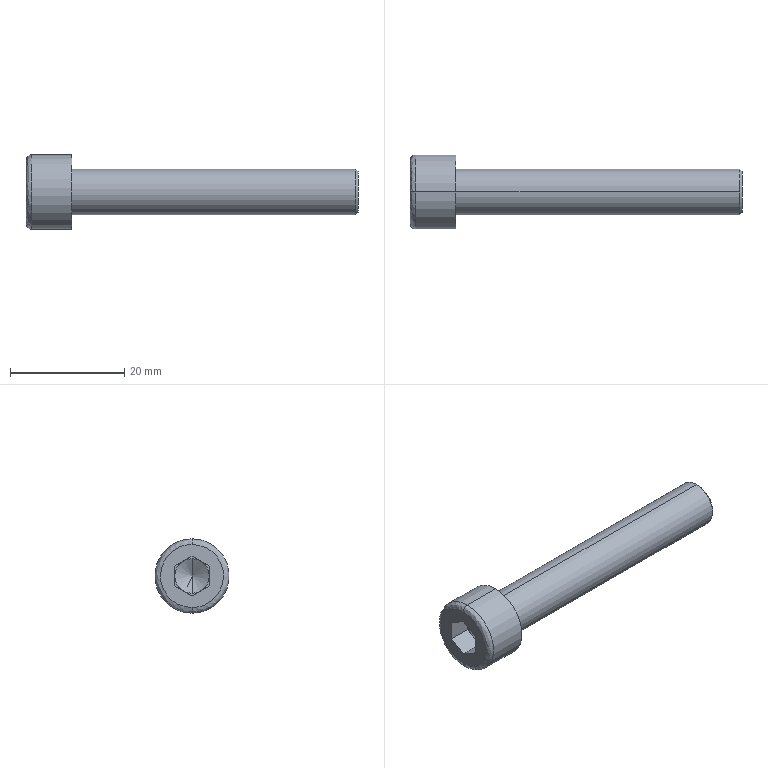Part | SolidWorks | features BaseBody 1 | 1 solid | 25 faces | box 58 x 13 x 13 mm | volume 3424 mm3 | plane 15 | cylinder 4 | cone 4 | spline 2 | commonest cylinder face diameters 8 x2 13 x2
STEP:
#1=CARTESIAN_POINT('',(1.,0.,6.5));
#2=VERTEX_POINT('',#1);
#3=CARTESIAN_POINT('',(1.,0.,-6.5));
#4=VERTEX_POINT('',#3);
#5=CARTESIAN_POINT('',(1.,0.,0.));
#6=DIRECTION('',(1.,0.,0.));
#7=DIRECTION('',(0.,0.,1.));
#8=AXIS2_PLACEMENT_3D('',#5,#6,#7);
#9=CIRCLE('',#8,6.5);
#10=EDGE_CURVE('',#2,#4,#9,.T.);
#11=ORIENTED_EDGE('',*,*,#10,.F.);
#12=CARTESIAN_POINT('',(0.,0.,5.5));
#13=VERTEX_POINT('',#12);
#14=CARTESIAN_POINT('',(1.,0.,5.5));
#15=DIRECTION('',(0.,-1.,0.));
#16=DIRECTION('',(0.,0.,1.));
#17=AXIS2_PLACEMENT_3D('',#14,#15,#16);
#18=CIRCLE('',#17,1.);
#19=EDGE_CURVE('',#2,#13,#18,.T.);
#20=ORIENTED_EDGE('',*,*,#19,.T.);
#21=CARTESIAN_POINT('',(0.,0.,-5.5));
#22=VERTEX_POINT('',#21);
#23=CARTESIAN_POINT('',(0.,0.,5.5));
#24=CARTESIAN_POINT('',(0.,-11.,5.5));
#25=CARTESIAN_POINT('',(0.,-11.,-5.5));
#26=CARTESIAN_POINT('',(0.,0.,-5.5));
#27=(BOUNDED_CURVE()B_SPLINE_CURVE(3,(#23,#24,#25,#26),.UNSPECIFIED.,.F.,.T.)B_SPLINE_CURVE_WITH_KNOTS((4,4),(0.,1.),.UNSPECIFIED.)CURVE()GEOMETRIC_REPRESENTATION_ITEM()RATIONAL_B_SPLINE_CURVE((1.,0.3333,0.3333,1.))REPRESENTATION_ITEM(''));
#28=EDGE_CURVE('',#13,#22,#27,.T.);
#29=ORIENTED_EDGE('',*,*,#28,.T.);
#30=CARTESIAN_POINT('',(1.,0.,-5.5));
#31=DIRECTION('',(0.,1.,0.));
#32=DIRECTION('',(0.,0.,-1.));
#33=AXIS2_PLACEMENT_3D('',#30,#31,#32);
#34=CIRCLE('',#33,1.);
#35=EDGE_CURVE('',#4,#22,#34,.T.);
#36=ORIENTED_EDGE('',*,*,#35,.F.);
#37=EDGE_LOOP('',(#11,#20,#29,#36));
#38=FACE_OUTER_BOUND('',#37,.T.);
#39=CARTESIAN_POINT('',(1.,0.,6.5));
#40=CARTESIAN_POINT('',(1.,-13.,6.5));
#41=CARTESIAN_POINT('',(1.,-13.,-6.5));
#42=CARTESIAN_POINT('',(1.,0.,-6.5));
#43=CARTESIAN_POINT('',(0.4142,0.,6.5));
#44=CARTESIAN_POINT('',(0.4142,-13.,6.5));
#45=CARTESIAN_POINT('',(0.4142,-13.,-6.5));
#46=CARTESIAN_POINT('',(0.4142,0.,-6.5));
#47=CARTESIAN_POINT('',(0.,0.,6.086));
#48=CARTESIAN_POINT('',(0.,-12.172,6.086));
#49=CARTESIAN_POINT('',(0.,-12.172,-6.086));
#50=CARTESIAN_POINT('',(0.,0.,-6.086));
#51=CARTESIAN_POINT('',(0.,0.,5.5));
#52=CARTESIAN_POINT('',(0.,-11.,5.5));
#53=CARTESIAN_POINT('',(0.,-11.,-5.5));
#54=CARTESIAN_POINT('',(0.,0.,-5.5));
#55=(BOUNDED_SURFACE()B_SPLINE_SURFACE(3,3,((#39,#40,#41,#42),(#43,#44,#45,#46),(#47,#48,#49,#50),(#51,#52,#53,#54)),.UNSPECIFIED.,.F.,.F.,.F.)B_SPLINE_SURFACE_WITH_KNOTS((4,4),(4,4),(0.,1.),(0.,1.),.UNSPECIFIED.)GEOMETRIC_REPRESENTATION_ITEM()RATIONAL_B_SPLINE_SURFACE(((1.,0.3333,0.3333,1.),(0.8047,0.2682,0.2682,0.8047),(0.8047,0.2682,0.2682,0.8047),(1.,0.3333,0.3333,1.)))REPRESENTATION_ITEM('')SURFACE());
#56=ADVANCED_FACE('',(#38),#55,.T.);
#57=CARTESIAN_POINT('',(57.6,0.,4.));
#58=VERTEX_POINT('',#57);
#59=CARTESIAN_POINT('',(57.6,0.,-4.));
#60=VERTEX_POINT('',#59);
#61=CARTESIAN_POINT('',(57.6,0.,0.));
#62=DIRECTION('',(-1.,0.,0.));
#63=DIRECTION('',(0.,0.,1.));
#64=AXIS2_PLACEMENT_3D('',#61,#62,#63);
#65=CIRCLE('',#64,4.);
#66=EDGE_CURVE('',#58,#60,#65,.T.);
#67=ORIENTED_EDGE('',*,*,#66,.T.);
#68=CARTESIAN_POINT('',(8.,0.,-4.));
#69=VERTEX_POINT('',#68);
#70=CARTESIAN_POINT('',(58.,0.,-4.));
#71=DIRECTION('',(-1.,0.,0.));
#72=VECTOR('',#71,1000.);
#73=LINE('',#70,#72);
#74=EDGE_CURVE('',#60,#69,#73,.T.);
#75=ORIENTED_EDGE('',*,*,#74,.T.);
#76=CARTESIAN_POINT('',(8.,0.,4.));
#77=VERTEX_POINT('',#76);
#78=CARTESIAN_POINT('',(8.,0.,0.));
#79=DIRECTION('',(1.,0.,0.));
#80=DIRECTION('',(0.,0.,1.));
#81=AXIS2_PLACEMENT_3D('',#78,#79,#80);
#82=CIRCLE('',#81,4.);
#83=EDGE_CURVE('',#69,#77,#82,.T.);
#84=ORIENTED_EDGE('',*,*,#83,.T.);
#85=CARTESIAN_POINT('',(58.,0.,4.));
#86=DIRECTION('',(-1.,0.,0.));
#87=VECTOR('',#86,1000.);
#88=LINE('',#85,#87);
#89=EDGE_CURVE('',#58,#77,#88,.T.);
#90=ORIENTED_EDGE('',*,*,#89,.F.);
#91=EDGE_LOOP('',(#67,#75,#84,#90));
#92=FACE_OUTER_BOUND('',#91,.T.);
#93=CARTESIAN_POINT('',(58.,0.,0.));
#94=DIRECTION('',(-1.,0.,0.));
#95=DIRECTION('',(0.,0.,1.));
#96=AXIS2_PLACEMENT_3D('',#93,#94,#95);
#97=CYLINDRICAL_SURFACE('',#96,4.);
#98=ADVANCED_FACE('',(#92),#97,.T.);
#99=CARTESIAN_POINT('',(58.,0.,3.6));
#100=VERTEX_POINT('',#99);
#101=CARTESIAN_POINT('',(58.,0.,-3.6));
#102=VERTEX_POINT('',#101);
#103=CARTESIAN_POINT('',(58.,0.,0.));
#104=DIRECTION('',(-1.,0.,0.));
#105=DIRECTION('',(0.,0.,1.));
#106=AXIS2_PLACEMENT_3D('',#103,#104,#105);
#107=CIRCLE('',#106,3.6);
#108=EDGE_CURVE('',#100,#102,#107,.T.);
#109=ORIENTED_EDGE('',*,*,#108,.T.);
#110=CARTESIAN_POINT('',(57.6,0.,-4.));
#111=DIRECTION('',(-0.7071,0.,-0.7071));
#112=VECTOR('',#111,1000.);
#113=LINE('',#110,#112);
#114=EDGE_CURVE('',#102,#60,#113,.T.);
#115=ORIENTED_EDGE('',*,*,#114,.T.);
#116=ORIENTED_EDGE('',*,*,#66,.F.);
#117=CARTESIAN_POINT('',(57.6,0.,4.));
#118=DIRECTION('',(-0.7071,0.,0.7071));
#119=VECTOR('',#118,1000.);
#120=LINE('',#117,#119);
#121=EDGE_CURVE('',#100,#58,#120,.T.);
#122=ORIENTED_EDGE('',*,*,#121,.F.);
#123=EDGE_LOOP('',(#109,#115,#116,#122));
#124=FACE_OUTER_BOUND('',#123,.T.);
#125=CARTESIAN_POINT('',(57.6,0.,0.));
#126=DIRECTION('',(-1.,0.,0.));
#127=DIRECTION('',(0.,0.,1.));
#128=AXIS2_PLACEMENT_3D('',#125,#126,#127);
#129=CONICAL_SURFACE('',#128,4.,0.7854);
#130=ADVANCED_FACE('',(#124),#129,.T.);
#131=CARTESIAN_POINT('',(8.,0.,-6.5));
#132=VERTEX_POINT('',#131);
#133=CARTESIAN_POINT('',(8.,0.,6.5));
#134=VERTEX_POINT('',#133);
#135=CARTESIAN_POINT('',(8.,0.,0.));
#136=DIRECTION('',(1.,0.,0.));
#137=DIRECTION('',(0.,0.,1.));
#138=AXIS2_PLACEMENT_3D('',#135,#136,#137);
#139=CIRCLE('',#138,6.5);
#140=EDGE_CURVE('',#132,#134,#139,.T.);
#141=ORIENTED_EDGE('',*,*,#140,.F.);
#142=CARTESIAN_POINT('',(8.,0.,-6.5));
#143=DIRECTION('',(-1.,0.,0.));
#144=VECTOR('',#143,1000.);
#145=LINE('',#142,#144);
#146=EDGE_CURVE('',#132,#4,#145,.T.);
#147=ORIENTED_EDGE('',*,*,#146,.T.);
#148=CARTESIAN_POINT('',(1.,0.,0.));
#149=DIRECTION('',(1.,0.,0.));
#150=DIRECTION('',(0.,0.,1.));
#151=AXIS2_PLACEMENT_3D('',#148,#149,#150);
#152=CIRCLE('',#151,6.5);
#153=EDGE_CURVE('',#4,#2,#152,.T.);
#154=ORIENTED_EDGE('',*,*,#153,.T.);
#155=CARTESIAN_POINT('',(8.,0.,6.5));
#156=DIRECTION('',(-1.,0.,0.));
#157=VECTOR('',#156,1000.);
#158=LINE('',#155,#157);
#159=EDGE_CURVE('',#134,#2,#158,.T.);
#160=ORIENTED_EDGE('',*,*,#159,.F.);
#161=EDGE_LOOP('',(#141,#147,#154,#160));
#162=FACE_OUTER_BOUND('',#161,.T.);
#163=CARTESIAN_POINT('',(8.,0.,0.));
#164=DIRECTION('',(-1.,0.,0.));
#165=DIRECTION('',(0.,0.,1.));
#166=AXIS2_PLACEMENT_3D('',#163,#164,#165);
#167=CYLINDRICAL_SURFACE('',#166,6.5);
#168=ADVANCED_FACE('',(#162),#167,.T.);
#169=CARTESIAN_POINT('',(5.732,0.,0.));
#170=VERTEX_POINT('',#169);
#171=CARTESIAN_POINT('',(4.,0.,3.));
#172=VERTEX_POINT('',#171);
#173=CARTESIAN_POINT('',(4.,0.,3.));
#174=DIRECTION('',(-0.5,0.,0.866));
#175=VECTOR('',#174,1000.);
#176=LINE('',#173,#175);
#177=EDGE_CURVE('',#170,#172,#176,.T.);
#178=ORIENTED_EDGE('',*,*,#177,.F.);
#179=CARTESIAN_POINT('',(4.,0.,-3.));
#180=VERTEX_POINT('',#179);
#181=CARTESIAN_POINT('',(4.,0.,-3.));
#182=DIRECTION('',(-0.5,0.,-0.866));
#183=VECTOR('',#182,1000.);
#184=LINE('',#181,#183);
#185=EDGE_CURVE('',#170,#180,#184,.T.);
#186=ORIENTED_EDGE('',*,*,#185,.T.);
#187=CARTESIAN_POINT('',(4.,-1.5,-2.598));
#188=VERTEX_POINT('',#187);
#189=CARTESIAN_POINT('',(4.,0.,0.));
#190=DIRECTION('',(1.,0.,0.));
#191=DIRECTION('',(0.,0.,1.));
#192=AXIS2_PLACEMENT_3D('',#189,#190,#191);
#193=CIRCLE('',#192,3.);
#194=EDGE_CURVE('',#188,#180,#193,.T.);
#195=ORIENTED_EDGE('',*,*,#194,.F.);
#196=CARTESIAN_POINT('',(4.,-3.,0.));
#197=VERTEX_POINT('',#196);
#198=CARTESIAN_POINT('',(4.,0.,0.));
#199=DIRECTION('',(-1.,0.,0.));
#200=DIRECTION('',(0.,0.,1.));
#201=AXIS2_PLACEMENT_3D('',#198,#199,#200);
#202=CIRCLE('',#201,3.);
#203=EDGE_CURVE('',#188,#197,#202,.T.);
#204=ORIENTED_EDGE('',*,*,#203,.T.);
#205=CARTESIAN_POINT('',(4.,-1.5,2.598));
#206=VERTEX_POINT('',#205);
#207=CARTESIAN_POINT('',(4.,0.,0.));
#208=DIRECTION('',(1.,0.,0.));
#209=DIRECTION('',(0.,0.,1.));
#210=AXIS2_PLACEMENT_3D('',#207,#208,#209);
#211=CIRCLE('',#210,3.);
#212=EDGE_CURVE('',#206,#197,#211,.T.);
#213=ORIENTED_EDGE('',*,*,#212,.F.);
#214=CARTESIAN_POINT('',(4.,0.,0.));
#215=DIRECTION('',(1.,0.,0.));
#216=DIRECTION('',(0.,0.,1.));
#217=AXIS2_PLACEMENT_3D('',#214,#215,#216);
#218=CIRCLE('',#217,3.);
#219=EDGE_CURVE('',#172,#206,#218,.T.);
#220=ORIENTED_EDGE('',*,*,#219,.F.);
#221=EDGE_LOOP('',(#178,#186,#195,#204,#213,#220));
#222=FACE_OUTER_BOUND('',#221,.T.);
#223=CARTESIAN_POINT('',(4.,0.,0.));
#224=DIRECTION('',(-1.,0.,0.));
#225=DIRECTION('',(0.,0.,1.));
#226=AXIS2_PLACEMENT_3D('',#223,#224,#225);
#227=CONICAL_SURFACE('',#226,3.,1.047);
#228=ADVANCED_FACE('',(#222),#227,.F.);
#229=ORIENTED_EDGE('',*,*,#74,.F.);
#230=CARTESIAN_POINT('',(57.6,0.,0.));
#231=DIRECTION('',(-1.,0.,0.));
#232=DIRECTION('',(0.,0.,1.));
#233=AXIS2_PLACEMENT_3D('',#230,#231,#232);
#234=CIRCLE('',#233,4.);
#235=EDGE_CURVE('',#60,#58,#234,.T.);
#236=ORIENTED_EDGE('',*,*,#235,.T.);
#237=ORIENTED_EDGE('',*,*,#89,.T.);
#238=CARTESIAN_POINT('',(8.,0.,0.));
#239=DIRECTION('',(1.,0.,0.));
#240=DIRECTION('',(0.,0.,1.));
#241=AXIS2_PLACEMENT_3D('',#238,#239,#240);
#242=CIRCLE('',#241,4.);
#243=EDGE_CURVE('',#77,#69,#242,.T.);
#244=ORIENTED_EDGE('',*,*,#243,.T.);
#245=EDGE_LOOP('',(#229,#236,#237,#244));
#246=FACE_OUTER_BOUND('',#245,.T.);
#247=CARTESIAN_POINT('',(58.,0.,0.));
#248=DIRECTION('',(-1.,0.,0.));
#249=DIRECTION('',(0.,0.,1.));
#250=AXIS2_PLACEMENT_3D('',#247,#248,#249);
#251=CYLINDRICAL_SURFACE('',#250,4.);
#252=ADVANCED_FACE('',(#246),#251,.T.);
#253=ORIENTED_EDGE('',*,*,#243,.F.);
#254=ORIENTED_EDGE('',*,*,#83,.F.);
#255=EDGE_LOOP('',(#253,#254));
#256=FACE_BOUND('',#255,.T.);
#257=CARTESIAN_POINT('',(8.,0.,0.));
#258=DIRECTION('',(1.,0.,0.));
#259=DIRECTION('',(0.,0.,1.));
#260=AXIS2_PLACEMENT_3D('',#257,#258,#259);
#261=CIRCLE('',#260,6.5);
#262=EDGE_CURVE('',#134,#132,#261,.T.);
#263=ORIENTED_EDGE('',*,*,#262,.T.);
#264=ORIENTED_EDGE('',*,*,#140,.T.);
#265=EDGE_LOOP('',(#263,#264));
#266=FACE_OUTER_BOUND('',#265,.T.);
#267=CARTESIAN_POINT('',(8.,0.,0.));
#268=DIRECTION('',(1.,0.,0.));
#269=DIRECTION('',(0.,0.,-1.));
#270=AXIS2_PLACEMENT_3D('',#267,#268,#269);
#271=PLANE('',#270);
#272=ADVANCED_FACE('',(#256,#266),#271,.T.);
#273=ORIENTED_EDGE('',*,*,#114,.F.);
#274=CARTESIAN_POINT('',(58.,0.,0.));
#275=DIRECTION('',(-1.,0.,0.));
#276=DIRECTION('',(0.,0.,1.));
#277=AXIS2_PLACEMENT_3D('',#274,#275,#276);
#278=CIRCLE('',#277,3.6);
#279=EDGE_CURVE('',#102,#100,#278,.T.);
#280=ORIENTED_EDGE('',*,*,#279,.T.);
#281=ORIENTED_EDGE('',*,*,#121,.T.);
#282=ORIENTED_EDGE('',*,*,#235,.F.);
#283=EDGE_LOOP('',(#273,#280,#281,#282));
#284=FACE_OUTER_BOUND('',#283,.T.);
#285=CARTESIAN_POINT('',(57.6,0.,0.));
#286=DIRECTION('',(-1.,0.,0.));
#287=DIRECTION('',(0.,0.,1.));
#288=AXIS2_PLACEMENT_3D('',#285,#286,#287);
#289=CONICAL_SURFACE('',#288,4.,0.7854);
#290=ADVANCED_FACE('',(#284),#289,.T.);
#291=ORIENTED_EDGE('',*,*,#146,.F.);
#292=ORIENTED_EDGE('',*,*,#262,.F.);
#293=ORIENTED_EDGE('',*,*,#159,.T.);
#294=ORIENTED_EDGE('',*,*,#10,.T.);
#295=EDGE_LOOP('',(#291,#292,#293,#294));
#296=FACE_OUTER_BOUND('',#295,.T.);
#297=CARTESIAN_POINT('',(8.,0.,0.));
#298=DIRECTION('',(-1.,0.,0.));
#299=DIRECTION('',(0.,0.,1.));
#300=AXIS2_PLACEMENT_3D('',#297,#298,#299);
#301=CYLINDRICAL_SURFACE('',#300,6.5);
#302=ADVANCED_FACE('',(#296),#301,.T.);
#303=ORIENTED_EDGE('',*,*,#108,.F.);
#304=ORIENTED_EDGE('',*,*,#279,.F.);
#305=EDGE_LOOP('',(#303,#304));
#306=FACE_OUTER_BOUND('',#305,.T.);
#307=CARTESIAN_POINT('',(58.,0.,0.));
#308=DIRECTION('',(1.,0.,0.));
#309=DIRECTION('',(0.,0.,-1.));
#310=AXIS2_PLACEMENT_3D('',#307,#308,#309);
#311=PLANE('',#310);
#312=ADVANCED_FACE('',(#306),#311,.T.);
#313=ORIENTED_EDGE('',*,*,#19,.F.);
#314=ORIENTED_EDGE('',*,*,#153,.F.);
#315=ORIENTED_EDGE('',*,*,#35,.T.);
#316=CARTESIAN_POINT('',(0.,0.,-5.5));
#317=CARTESIAN_POINT('',(0.,11.,-5.5));
#318=CARTESIAN_POINT('',(0.,11.,5.5));
#319=CARTESIAN_POINT('',(0.,0.,5.5));
#320=(BOUNDED_CURVE()B_SPLINE_CURVE(3,(#316,#317,#318,#319),.UNSPECIFIED.,.F.,.T.)B_SPLINE_CURVE_WITH_KNOTS((4,4),(0.,1.),.UNSPECIFIED.)CURVE()GEOMETRIC_REPRESENTATION_ITEM()RATIONAL_B_SPLINE_CURVE((1.,0.3333,0.3333,1.))REPRESENTATION_ITEM(''));
#321=EDGE_CURVE('',#22,#13,#320,.T.);
#322=ORIENTED_EDGE('',*,*,#321,.T.);
#323=EDGE_LOOP('',(#313,#314,#315,#322));
#324=FACE_OUTER_BOUND('',#323,.T.);
#325=CARTESIAN_POINT('',(1.,0.,-6.5));
#326=CARTESIAN_POINT('',(1.,13.,-6.5));
#327=CARTESIAN_POINT('',(1.,13.,6.5));
#328=CARTESIAN_POINT('',(1.,0.,6.5));
#329=CARTESIAN_POINT('',(0.4142,0.,-6.5));
#330=CARTESIAN_POINT('',(0.4142,13.,-6.5));
#331=CARTESIAN_POINT('',(0.4142,13.,6.5));
#332=CARTESIAN_POINT('',(0.4142,0.,6.5));
#333=CARTESIAN_POINT('',(0.,0.,-6.086));
#334=CARTESIAN_POINT('',(0.,12.172,-6.086));
#335=CARTESIAN_POINT('',(0.,12.172,6.086));
#336=CARTESIAN_POINT('',(0.,0.,6.086));
#337=CARTESIAN_POINT('',(0.,0.,-5.5));
#338=CARTESIAN_POINT('',(0.,11.,-5.5));
#339=CARTESIAN_POINT('',(0.,11.,5.5));
#340=CARTESIAN_POINT('',(0.,0.,5.5));
#341=(BOUNDED_SURFACE()B_SPLINE_SURFACE(3,3,((#325,#326,#327,#328),(#329,#330,#331,#332),(#333,#334,#335,#336),(#337,#338,#339,#340)),.UNSPECIFIED.,.F.,.F.,.T.)B_SPLINE_SURFACE_WITH_KNOTS((4,4),(4,4),(0.,1.),(0.,1.),.UNSPECIFIED.)GEOMETRIC_REPRESENTATION_ITEM()RATIONAL_B_SPLINE_SURFACE(((1.,0.3333,0.3333,1.),(0.8047,0.2682,0.2682,0.8047),(0.8047,0.2682,0.2682,0.8047),(1.,0.3333,0.3333,1.)))REPRESENTATION_ITEM('')SURFACE());
#342=ADVANCED_FACE('',(#324),#341,.T.);
#343=CARTESIAN_POINT('',(0.,3.,1.732));
#344=VERTEX_POINT('',#343);
#345=CARTESIAN_POINT('',(0.,3.,-1.732));
#346=VERTEX_POINT('',#345);
#347=CARTESIAN_POINT('',(0.,3.,0.));
#348=DIRECTION('',(0.,0.,-1.));
#349=VECTOR('',#348,1000.);
#350=LINE('',#347,#349);
#351=EDGE_CURVE('',#344,#346,#350,.T.);
#352=ORIENTED_EDGE('',*,*,#351,.F.);
#353=CARTESIAN_POINT('',(0.,0.,3.464));
#354=VERTEX_POINT('',#353);
#355=CARTESIAN_POINT('',(0.,0.,3.464));
#356=DIRECTION('',(0.,0.866,-0.5));
#357=VECTOR('',#356,1000.);
#358=LINE('',#355,#357);
#359=EDGE_CURVE('',#354,#344,#358,.T.);
#360=ORIENTED_EDGE('',*,*,#359,.F.);
#361=CARTESIAN_POINT('',(0.,-3.,1.732));
#362=VERTEX_POINT('',#361);
#363=CARTESIAN_POINT('',(0.,-3.,1.732));
#364=DIRECTION('',(0.,0.866,0.5));
#365=VECTOR('',#364,1000.);
#366=LINE('',#363,#365);
#367=EDGE_CURVE('',#362,#354,#366,.T.);
#368=ORIENTED_EDGE('',*,*,#367,.F.);
#369=CARTESIAN_POINT('',(0.,-3.,-1.732));
#370=VERTEX_POINT('',#369);
#371=CARTESIAN_POINT('',(0.,-3.,0.));
#372=DIRECTION('',(0.,0.,1.));
#373=VECTOR('',#372,1000.);
#374=LINE('',#371,#373);
#375=EDGE_CURVE('',#370,#362,#374,.T.);
#376=ORIENTED_EDGE('',*,*,#375,.F.);
#377=CARTESIAN_POINT('',(0.,0.,-3.464));
#378=VERTEX_POINT('',#377);
#379=CARTESIAN_POINT('',(0.,0.,-3.464));
#380=DIRECTION('',(0.,-0.866,0.5));
#381=VECTOR('',#380,1000.);
#382=LINE('',#379,#381);
#383=EDGE_CURVE('',#378,#370,#382,.T.);
#384=ORIENTED_EDGE('',*,*,#383,.F.);
#385=CARTESIAN_POINT('',(0.,3.,-1.732));
#386=DIRECTION('',(0.,-0.866,-0.5));
#387=VECTOR('',#386,1000.);
#388=LINE('',#385,#387);
#389=EDGE_CURVE('',#346,#378,#388,.T.);
#390=ORIENTED_EDGE('',*,*,#389,.F.);
#391=EDGE_LOOP('',(#352,#360,#368,#376,#384,#390));
#392=FACE_BOUND('',#391,.T.);
#393=ORIENTED_EDGE('',*,*,#28,.F.);
#394=ORIENTED_EDGE('',*,*,#321,.F.);
#395=EDGE_LOOP('',(#393,#394));
#396=FACE_OUTER_BOUND('',#395,.T.);
#397=CARTESIAN_POINT('',(0.,0.,0.));
#398=DIRECTION('',(1.,0.,0.));
#399=DIRECTION('',(0.,0.,-1.));
#400=AXIS2_PLACEMENT_3D('',#397,#398,#399);
#401=PLANE('',#400);
#402=ADVANCED_FACE('',(#392,#396),#401,.F.);
#403=CARTESIAN_POINT('',(4.,3.,-1.732));
#404=VERTEX_POINT('',#403);
#405=CARTESIAN_POINT('',(4.,3.,-1.732));
#406=DIRECTION('',(-1.,0.,0.));
#407=VECTOR('',#406,1000.);
#408=LINE('',#405,#407);
#409=EDGE_CURVE('',#404,#346,#408,.T.);
#410=ORIENTED_EDGE('',*,*,#409,.T.);
#411=ORIENTED_EDGE('',*,*,#389,.T.);
#412=CARTESIAN_POINT('',(4.,0.,-3.464));
#413=VERTEX_POINT('',#412);
#414=CARTESIAN_POINT('',(4.,0.,-3.464));
#415=DIRECTION('',(1.,0.,0.));
#416=VECTOR('',#415,1000.);
#417=LINE('',#414,#416);
#418=EDGE_CURVE('',#378,#413,#417,.T.);
#419=ORIENTED_EDGE('',*,*,#418,.T.);
#420=CARTESIAN_POINT('',(4.,1.5,-2.598));
#421=VERTEX_POINT('',#420);
#422=CARTESIAN_POINT('',(4.,0.,-3.464));
#423=DIRECTION('',(0.,0.866,0.5));
#424=VECTOR('',#423,1000.);
#425=LINE('',#422,#424);
#426=EDGE_CURVE('',#413,#421,#425,.T.);
#427=ORIENTED_EDGE('',*,*,#426,.T.);
#428=CARTESIAN_POINT('',(4.,1.5,-2.598));
#429=DIRECTION('',(0.,0.866,0.5));
#430=VECTOR('',#429,1000.);
#431=LINE('',#428,#430);
#432=EDGE_CURVE('',#421,#404,#431,.T.);
#433=ORIENTED_EDGE('',*,*,#432,.T.);
#434=EDGE_LOOP('',(#410,#411,#419,#427,#433));
#435=FACE_OUTER_BOUND('',#434,.T.);
#436=CARTESIAN_POINT('',(4.,0.,-3.464));
#437=DIRECTION('',(0.,-0.5,0.866));
#438=DIRECTION('',(0.,-0.866,-0.5));
#439=AXIS2_PLACEMENT_3D('',#436,#437,#438);
#440=PLANE('',#439);
#441=ADVANCED_FACE('',(#435),#440,.T.);
#442=CARTESIAN_POINT('',(4.,3.,1.732));
#443=VERTEX_POINT('',#442);
#444=CARTESIAN_POINT('',(4.,3.,1.732));
#445=DIRECTION('',(-1.,0.,0.));
#446=VECTOR('',#445,1000.);
#447=LINE('',#444,#446);
#448=EDGE_CURVE('',#443,#344,#447,.T.);
#449=ORIENTED_EDGE('',*,*,#448,.T.);
#450=ORIENTED_EDGE('',*,*,#351,.T.);
#451=ORIENTED_EDGE('',*,*,#409,.F.);
#452=CARTESIAN_POINT('',(4.,3.,0.));
#453=VERTEX_POINT('',#452);
#454=CARTESIAN_POINT('',(4.,3.,-3.464));
#455=DIRECTION('',(0.,0.,1.));
#456=VECTOR('',#455,1000.);
#457=LINE('',#454,#456);
#458=EDGE_CURVE('',#404,#453,#457,.T.);
#459=ORIENTED_EDGE('',*,*,#458,.T.);
#460=CARTESIAN_POINT('',(4.,3.,-3.464));
#461=DIRECTION('',(0.,0.,1.));
#462=VECTOR('',#461,1000.);
#463=LINE('',#460,#462);
#464=EDGE_CURVE('',#453,#443,#463,.T.);
#465=ORIENTED_EDGE('',*,*,#464,.T.);
#466=EDGE_LOOP('',(#449,#450,#451,#459,#465));
#467=FACE_OUTER_BOUND('',#466,.T.);
#468=CARTESIAN_POINT('',(4.,3.,-1.732));
#469=DIRECTION('',(0.,-1.,0.));
#470=DIRECTION('',(0.,0.,-1.));
#471=AXIS2_PLACEMENT_3D('',#468,#469,#470);
#472=PLANE('',#471);
#473=ADVANCED_FACE('',(#467),#472,.T.);
#474=CARTESIAN_POINT('',(4.,0.,3.464));
#475=VERTEX_POINT('',#474);
#476=CARTESIAN_POINT('',(4.,0.,3.464));
#477=DIRECTION('',(-1.,0.,0.));
#478=VECTOR('',#477,1000.);
#479=LINE('',#476,#478);
#480=EDGE_CURVE('',#475,#354,#479,.T.);
#481=ORIENTED_EDGE('',*,*,#480,.T.);
#482=ORIENTED_EDGE('',*,*,#359,.T.);
#483=ORIENTED_EDGE('',*,*,#448,.F.);
#484=CARTESIAN_POINT('',(4.,1.5,2.598));
#485=VERTEX_POINT('',#484);
#486=CARTESIAN_POINT('',(4.,3.,1.732));
#487=DIRECTION('',(0.,-0.866,0.5));
#488=VECTOR('',#487,1000.);
#489=LINE('',#486,#488);
#490=EDGE_CURVE('',#443,#485,#489,.T.);
#491=ORIENTED_EDGE('',*,*,#490,.T.);
#492=CARTESIAN_POINT('',(4.,3.,1.732));
#493=DIRECTION('',(0.,-0.866,0.5));
#494=VECTOR('',#493,1000.);
#495=LINE('',#492,#494);
#496=EDGE_CURVE('',#485,#475,#495,.T.);
#497=ORIENTED_EDGE('',*,*,#496,.T.);
#498=EDGE_LOOP('',(#481,#482,#483,#491,#497));
#499=FACE_OUTER_BOUND('',#498,.T.);
#500=CARTESIAN_POINT('',(4.,3.,1.732));
#501=DIRECTION('',(0.,-0.5,-0.866));
#502=DIRECTION('',(0.,0.866,-0.5));
#503=AXIS2_PLACEMENT_3D('',#500,#501,#502);
#504=PLANE('',#503);
#505=ADVANCED_FACE('',(#499),#504,.T.);
#506=CARTESIAN_POINT('',(4.,-3.,1.732));
#507=VERTEX_POINT('',#506);
#508=CARTESIAN_POINT('',(4.,-3.,1.732));
#509=DIRECTION('',(-1.,0.,0.));
#510=VECTOR('',#509,1000.);
#511=LINE('',#508,#510);
#512=EDGE_CURVE('',#507,#362,#511,.T.);
#513=ORIENTED_EDGE('',*,*,#512,.T.);
#514=ORIENTED_EDGE('',*,*,#367,.T.);
#515=ORIENTED_EDGE('',*,*,#480,.F.);
#516=CARTESIAN_POINT('',(4.,0.,3.464));
#517=DIRECTION('',(0.,-0.866,-0.5));
#518=VECTOR('',#517,1000.);
#519=LINE('',#516,#518);
#520=EDGE_CURVE('',#475,#206,#519,.T.);
#521=ORIENTED_EDGE('',*,*,#520,.T.);
#522=CARTESIAN_POINT('',(4.,-1.5,2.598));
#523=DIRECTION('',(0.,-0.866,-0.5));
#524=VECTOR('',#523,1000.);
#525=LINE('',#522,#524);
#526=EDGE_CURVE('',#206,#507,#525,.T.);
#527=ORIENTED_EDGE('',*,*,#526,.T.);
#528=EDGE_LOOP('',(#513,#514,#515,#521,#527));
#529=FACE_OUTER_BOUND('',#528,.T.);
#530=CARTESIAN_POINT('',(4.,0.,3.464));
#531=DIRECTION('',(0.,0.5,-0.866));
#532=DIRECTION('',(0.,0.866,0.5));
#533=AXIS2_PLACEMENT_3D('',#530,#531,#532);
#534=PLANE('',#533);
#535=ADVANCED_FACE('',(#529),#534,.T.);
#536=CARTESIAN_POINT('',(4.,-3.,-1.732));
#537=VERTEX_POINT('',#536);
#538=CARTESIAN_POINT('',(4.,-3.,-1.732));
#539=DIRECTION('',(-1.,0.,0.));
#540=VECTOR('',#539,1000.);
#541=LINE('',#538,#540);
#542=EDGE_CURVE('',#537,#370,#541,.T.);
#543=ORIENTED_EDGE('',*,*,#542,.T.);
#544=ORIENTED_EDGE('',*,*,#375,.T.);
#545=ORIENTED_EDGE('',*,*,#512,.F.);
#546=CARTESIAN_POINT('',(4.,-3.,-3.464));
#547=DIRECTION('',(0.,0.,-1.));
#548=VECTOR('',#547,1000.);
#549=LINE('',#546,#548);
#550=EDGE_CURVE('',#507,#197,#549,.T.);
#551=ORIENTED_EDGE('',*,*,#550,.T.);
#552=CARTESIAN_POINT('',(4.,-3.,1.732));
#553=DIRECTION('',(0.,0.,-1.));
#554=VECTOR('',#553,1000.);
#555=LINE('',#552,#554);
#556=EDGE_CURVE('',#197,#537,#555,.T.);
#557=ORIENTED_EDGE('',*,*,#556,.T.);
#558=EDGE_LOOP('',(#543,#544,#545,#551,#557));
#559=FACE_OUTER_BOUND('',#558,.T.);
#560=CARTESIAN_POINT('',(4.,-3.,1.732));
#561=DIRECTION('',(0.,1.,0.));
#562=DIRECTION('',(0.,0.,1.));
#563=AXIS2_PLACEMENT_3D('',#560,#561,#562);
#564=PLANE('',#563);
#565=ADVANCED_FACE('',(#559),#564,.T.);
#566=ORIENTED_EDGE('',*,*,#418,.F.);
#567=ORIENTED_EDGE('',*,*,#383,.T.);
#568=ORIENTED_EDGE('',*,*,#542,.F.);
#569=CARTESIAN_POINT('',(4.,-3.,-1.732));
#570=DIRECTION('',(0.,0.866,-0.5));
#571=VECTOR('',#570,1000.);
#572=LINE('',#569,#571);
#573=EDGE_CURVE('',#537,#188,#572,.T.);
#574=ORIENTED_EDGE('',*,*,#573,.T.);
#575=CARTESIAN_POINT('',(4.,-3.,-1.732));
#576=DIRECTION('',(0.,0.866,-0.5));
#577=VECTOR('',#576,1000.);
#578=LINE('',#575,#577);
#579=EDGE_CURVE('',#188,#413,#578,.T.);
#580=ORIENTED_EDGE('',*,*,#579,.T.);
#581=EDGE_LOOP('',(#566,#567,#568,#574,#580));
#582=FACE_OUTER_BOUND('',#581,.T.);
#583=CARTESIAN_POINT('',(4.,-3.,-1.732));
#584=DIRECTION('',(0.,0.5,0.866));
#585=DIRECTION('',(0.,-0.866,0.5));
#586=AXIS2_PLACEMENT_3D('',#583,#584,#585);
#587=PLANE('',#586);
#588=ADVANCED_FACE('',(#582),#587,.T.);
#589=ORIENTED_EDGE('',*,*,#579,.F.);
#590=ORIENTED_EDGE('',*,*,#194,.T.);
#591=CARTESIAN_POINT('',(4.,0.,0.));
#592=DIRECTION('',(1.,0.,0.));
#593=DIRECTION('',(0.,0.,1.));
#594=AXIS2_PLACEMENT_3D('',#591,#592,#593);
#595=CIRCLE('',#594,3.);
#596=EDGE_CURVE('',#180,#421,#595,.T.);
#597=ORIENTED_EDGE('',*,*,#596,.T.);
#598=ORIENTED_EDGE('',*,*,#426,.F.);
#599=EDGE_LOOP('',(#589,#590,#597,#598));
#600=FACE_OUTER_BOUND('',#599,.T.);
#601=CARTESIAN_POINT('',(4.,0.,-3.464));
#602=DIRECTION('',(1.,0.,0.));
#603=DIRECTION('',(0.,0.,-1.));
#604=AXIS2_PLACEMENT_3D('',#601,#602,#603);
#605=PLANE('',#604);
#606=ADVANCED_FACE('',(#600),#605,.F.);
#607=ORIENTED_EDGE('',*,*,#496,.F.);
#608=CARTESIAN_POINT('',(4.,0.,0.));
#609=DIRECTION('',(1.,0.,0.));
#610=DIRECTION('',(0.,0.,1.));
#611=AXIS2_PLACEMENT_3D('',#608,#609,#610);
#612=CIRCLE('',#611,3.);
#613=EDGE_CURVE('',#485,#172,#612,.T.);
#614=ORIENTED_EDGE('',*,*,#613,.T.);
#615=ORIENTED_EDGE('',*,*,#219,.T.);
#616=ORIENTED_EDGE('',*,*,#520,.F.);
#617=EDGE_LOOP('',(#607,#614,#615,#616));
#618=FACE_OUTER_BOUND('',#617,.T.);
#619=CARTESIAN_POINT('',(4.,0.,-3.464));
#620=DIRECTION('',(1.,0.,0.));
#621=DIRECTION('',(0.,0.,-1.));
#622=AXIS2_PLACEMENT_3D('',#619,#620,#621);
#623=PLANE('',#622);
#624=ADVANCED_FACE('',(#618),#623,.F.);
#625=ORIENTED_EDGE('',*,*,#556,.F.);
#626=ORIENTED_EDGE('',*,*,#203,.F.);
#627=ORIENTED_EDGE('',*,*,#573,.F.);
#628=EDGE_LOOP('',(#625,#626,#627));
#629=FACE_OUTER_BOUND('',#628,.T.);
#630=CARTESIAN_POINT('',(4.,0.,-3.464));
#631=DIRECTION('',(1.,0.,0.));
#632=DIRECTION('',(0.,0.,-1.));
#633=AXIS2_PLACEMENT_3D('',#630,#631,#632);
#634=PLANE('',#633);
#635=ADVANCED_FACE('',(#629),#634,.F.);
#636=ORIENTED_EDGE('',*,*,#185,.F.);
#637=ORIENTED_EDGE('',*,*,#177,.T.);
#638=ORIENTED_EDGE('',*,*,#613,.F.);
#639=CARTESIAN_POINT('',(4.,0.,0.));
#640=DIRECTION('',(1.,0.,0.));
#641=DIRECTION('',(0.,0.,1.));
#642=AXIS2_PLACEMENT_3D('',#639,#640,#641);
#643=CIRCLE('',#642,3.);
#644=EDGE_CURVE('',#453,#485,#643,.T.);
#645=ORIENTED_EDGE('',*,*,#644,.F.);
#646=CARTESIAN_POINT('',(4.,0.,0.));
#647=DIRECTION('',(1.,0.,0.));
#648=DIRECTION('',(0.,0.,1.));
#649=AXIS2_PLACEMENT_3D('',#646,#647,#648);
#650=CIRCLE('',#649,3.);
#651=EDGE_CURVE('',#421,#453,#650,.T.);
#652=ORIENTED_EDGE('',*,*,#651,.F.);
#653=ORIENTED_EDGE('',*,*,#596,.F.);
#654=EDGE_LOOP('',(#636,#637,#638,#645,#652,#653));
#655=FACE_OUTER_BOUND('',#654,.T.);
#656=CARTESIAN_POINT('',(4.,0.,0.));
#657=DIRECTION('',(-1.,0.,0.));
#658=DIRECTION('',(0.,0.,1.));
#659=AXIS2_PLACEMENT_3D('',#656,#657,#658);
#660=CONICAL_SURFACE('',#659,3.,1.047);
#661=ADVANCED_FACE('',(#655),#660,.F.);
#662=ORIENTED_EDGE('',*,*,#526,.F.);
#663=ORIENTED_EDGE('',*,*,#212,.T.);
#664=ORIENTED_EDGE('',*,*,#550,.F.);
#665=EDGE_LOOP('',(#662,#663,#664));
#666=FACE_OUTER_BOUND('',#665,.T.);
#667=CARTESIAN_POINT('',(4.,0.,-3.464));
#668=DIRECTION('',(1.,0.,0.));
#669=DIRECTION('',(0.,0.,-1.));
#670=AXIS2_PLACEMENT_3D('',#667,#668,#669);
#671=PLANE('',#670);
#672=ADVANCED_FACE('',(#666),#671,.F.);
#673=ORIENTED_EDGE('',*,*,#464,.F.);
#674=ORIENTED_EDGE('',*,*,#644,.T.);
#675=ORIENTED_EDGE('',*,*,#490,.F.);
#676=EDGE_LOOP('',(#673,#674,#675));
#677=FACE_OUTER_BOUND('',#676,.T.);
#678=CARTESIAN_POINT('',(4.,0.,-3.464));
#679=DIRECTION('',(1.,0.,0.));
#680=DIRECTION('',(0.,0.,-1.));
#681=AXIS2_PLACEMENT_3D('',#678,#679,#680);
#682=PLANE('',#681);
#683=ADVANCED_FACE('',(#677),#682,.F.);
#684=ORIENTED_EDGE('',*,*,#432,.F.);
#685=ORIENTED_EDGE('',*,*,#651,.T.);
#686=ORIENTED_EDGE('',*,*,#458,.F.);
#687=EDGE_LOOP('',(#684,#685,#686));
#688=FACE_OUTER_BOUND('',#687,.T.);
#689=CARTESIAN_POINT('',(4.,0.,-3.464));
#690=DIRECTION('',(1.,0.,0.));
#691=DIRECTION('',(0.,0.,-1.));
#692=AXIS2_PLACEMENT_3D('',#689,#690,#691);
#693=PLANE('',#692);
#694=ADVANCED_FACE('',(#688),#693,.F.);
#695=CLOSED_SHELL('',(#56,#98,#130,#168,#228,#252,#272,#290,#302,#312,#342,#402,#441,#473,#505,#535,#565,#588,#606,#624,#635,#661,#672,#683,#694));
#696=MANIFOLD_SOLID_BREP('',#695);
#697=CARTESIAN_POINT('',(0.,0.,0.));
#698=DIRECTION('',(0.,0.,1.));
#699=DIRECTION('',(1.,0.,0.));
#700=AXIS2_PLACEMENT_3D('',#697,#698,#699);
#701=(LENGTH_UNIT()NAMED_UNIT(*)SI_UNIT(.MILLI.,.METRE.));
#702=UNCERTAINTY_MEASURE_WITH_UNIT(LENGTH_MEASURE(0.00001),#701,'','');
#703=(NAMED_UNIT(*)PLANE_ANGLE_UNIT()SI_UNIT($,.RADIAN.));
#704=(NAMED_UNIT(*)SI_UNIT($,.STERADIAN.)SOLID_ANGLE_UNIT());
#705=(GEOMETRIC_REPRESENTATION_CONTEXT(3)GLOBAL_UNCERTAINTY_ASSIGNED_CONTEXT((#702))GLOBAL_UNIT_ASSIGNED_CONTEXT((#701,#703,#704))REPRESENTATION_CONTEXT('',''));
#706=ADVANCED_BREP_SHAPE_REPRESENTATION('',(#696,#700),#705);